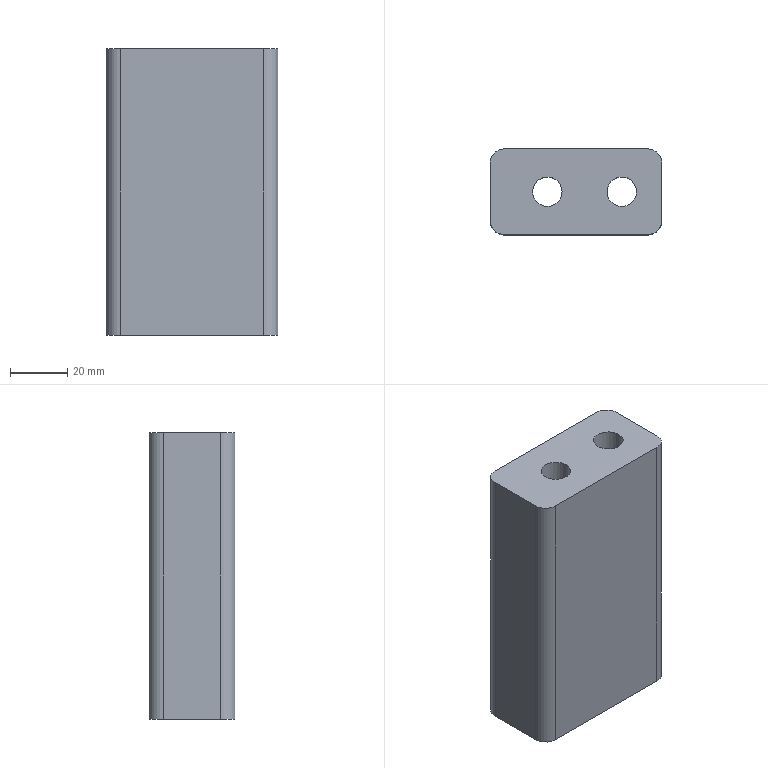Part | NX | features 8 2 | 1 solid | 16 faces | box 60 x 30 x 100 mm | volume 137229 mm3 | plane 8 | cylinder 8 | commonest cylinder face diameters 10 x4 10.3 x2 18 x2
STEP:
#1=CARTESIAN_POINT('',(3731.649,-412.84,91.));
#2=VERTEX_POINT('',#1);
#3=CARTESIAN_POINT('',(3726.499,-412.84,91.));
#4=DIRECTION('',(0.,0.,-1.));
#5=DIRECTION('',(1.,0.,0.));
#6=AXIS2_PLACEMENT_3D('',#3,#4,#5);
#7=CIRCLE('',#6,5.15);
#8=EDGE_CURVE('',#2,#2,#7,.T.);
#9=ORIENTED_EDGE('',*,*,#8,.T.);
#10=EDGE_LOOP('',(#9));
#11=FACE_BOUND('',#10,.T.);
#12=CARTESIAN_POINT('',(3711.499,-397.84,91.));
#13=VERTEX_POINT('',#12);
#14=CARTESIAN_POINT('',(3761.499,-397.84,91.));
#15=VERTEX_POINT('',#14);
#16=CARTESIAN_POINT('',(3721.499,-397.84,91.));
#17=DIRECTION('',(1.,0.,0.));
#18=VECTOR('',#17,1000.);
#19=LINE('',#16,#18);
#20=EDGE_CURVE('',#13,#15,#19,.T.);
#21=ORIENTED_EDGE('',*,*,#20,.F.);
#22=CARTESIAN_POINT('',(3706.499,-402.84,91.));
#23=VERTEX_POINT('',#22);
#24=CARTESIAN_POINT('',(3711.499,-402.84,91.));
#25=DIRECTION('',(0.,0.,1.));
#26=DIRECTION('',(1.,0.,0.));
#27=AXIS2_PLACEMENT_3D('',#24,#25,#26);
#28=CIRCLE('',#27,5.);
#29=EDGE_CURVE('',#13,#23,#28,.T.);
#30=ORIENTED_EDGE('',*,*,#29,.T.);
#31=CARTESIAN_POINT('',(3706.499,-422.84,91.));
#32=VERTEX_POINT('',#31);
#33=CARTESIAN_POINT('',(3706.499,-412.84,91.));
#34=DIRECTION('',(0.,1.,0.));
#35=VECTOR('',#34,1000.);
#36=LINE('',#33,#35);
#37=EDGE_CURVE('',#32,#23,#36,.T.);
#38=ORIENTED_EDGE('',*,*,#37,.F.);
#39=CARTESIAN_POINT('',(3711.499,-427.84,91.));
#40=VERTEX_POINT('',#39);
#41=CARTESIAN_POINT('',(3711.499,-422.84,91.));
#42=DIRECTION('',(0.,0.,1.));
#43=DIRECTION('',(1.,0.,0.));
#44=AXIS2_PLACEMENT_3D('',#41,#42,#43);
#45=CIRCLE('',#44,5.);
#46=EDGE_CURVE('',#32,#40,#45,.T.);
#47=ORIENTED_EDGE('',*,*,#46,.T.);
#48=CARTESIAN_POINT('',(3761.499,-427.84,91.));
#49=VERTEX_POINT('',#48);
#50=CARTESIAN_POINT('',(3721.499,-427.84,91.));
#51=DIRECTION('',(-1.,0.,0.));
#52=VECTOR('',#51,1000.);
#53=LINE('',#50,#52);
#54=EDGE_CURVE('',#49,#40,#53,.T.);
#55=ORIENTED_EDGE('',*,*,#54,.F.);
#56=CARTESIAN_POINT('',(3766.499,-422.84,91.));
#57=VERTEX_POINT('',#56);
#58=CARTESIAN_POINT('',(3761.499,-422.84,91.));
#59=DIRECTION('',(0.,0.,1.));
#60=DIRECTION('',(1.,0.,0.));
#61=AXIS2_PLACEMENT_3D('',#58,#59,#60);
#62=CIRCLE('',#61,5.);
#63=EDGE_CURVE('',#49,#57,#62,.T.);
#64=ORIENTED_EDGE('',*,*,#63,.T.);
#65=CARTESIAN_POINT('',(3766.499,-402.84,91.));
#66=VERTEX_POINT('',#65);
#67=CARTESIAN_POINT('',(3766.499,-412.84,91.));
#68=DIRECTION('',(0.,-1.,0.));
#69=VECTOR('',#68,1000.);
#70=LINE('',#67,#69);
#71=EDGE_CURVE('',#66,#57,#70,.T.);
#72=ORIENTED_EDGE('',*,*,#71,.F.);
#73=CARTESIAN_POINT('',(3761.499,-402.84,91.));
#74=DIRECTION('',(0.,0.,1.));
#75=DIRECTION('',(1.,0.,0.));
#76=AXIS2_PLACEMENT_3D('',#73,#74,#75);
#77=CIRCLE('',#76,5.);
#78=EDGE_CURVE('',#66,#15,#77,.T.);
#79=ORIENTED_EDGE('',*,*,#78,.T.);
#80=EDGE_LOOP('',(#21,#30,#38,#47,#55,#64,#72,#79));
#81=FACE_BOUND('',#80,.T.);
#82=CARTESIAN_POINT('',(3757.649,-412.84,91.));
#83=VERTEX_POINT('',#82);
#84=CARTESIAN_POINT('',(3752.499,-412.84,91.));
#85=DIRECTION('',(0.,0.,-1.));
#86=DIRECTION('',(1.,0.,0.));
#87=AXIS2_PLACEMENT_3D('',#84,#85,#86);
#88=CIRCLE('',#87,5.15);
#89=EDGE_CURVE('',#83,#83,#88,.T.);
#90=ORIENTED_EDGE('',*,*,#89,.T.);
#91=EDGE_LOOP('',(#90));
#92=FACE_BOUND('',#91,.T.);
#93=CARTESIAN_POINT('',(3721.499,-412.84,91.));
#94=DIRECTION('',(0.,0.,1.));
#95=DIRECTION('',(-1.,0.,0.));
#96=AXIS2_PLACEMENT_3D('',#93,#94,#95);
#97=PLANE('',#96);
#98=ADVANCED_FACE('',(#11,#81,#92),#97,.T.);
#99=CARTESIAN_POINT('',(3735.499,-412.84,-9.));
#100=VERTEX_POINT('',#99);
#101=CARTESIAN_POINT('',(3726.499,-412.84,-9.));
#102=DIRECTION('',(0.,0.,1.));
#103=DIRECTION('',(1.,0.,0.));
#104=AXIS2_PLACEMENT_3D('',#101,#102,#103);
#105=CIRCLE('',#104,9.);
#106=EDGE_CURVE('',#100,#100,#105,.T.);
#107=ORIENTED_EDGE('',*,*,#106,.T.);
#108=EDGE_LOOP('',(#107));
#109=FACE_BOUND('',#108,.T.);
#110=CARTESIAN_POINT('',(3706.499,-402.84,-9.));
#111=VERTEX_POINT('',#110);
#112=CARTESIAN_POINT('',(3706.499,-422.84,-9.));
#113=VERTEX_POINT('',#112);
#114=CARTESIAN_POINT('',(3706.499,-412.84,-9.));
#115=DIRECTION('',(0.,-1.,0.));
#116=VECTOR('',#115,1000.);
#117=LINE('',#114,#116);
#118=EDGE_CURVE('',#111,#113,#117,.T.);
#119=ORIENTED_EDGE('',*,*,#118,.F.);
#120=CARTESIAN_POINT('',(3711.499,-397.84,-9.));
#121=VERTEX_POINT('',#120);
#122=CARTESIAN_POINT('',(3711.499,-402.84,-9.));
#123=DIRECTION('',(0.,0.,-1.));
#124=DIRECTION('',(-1.,0.,0.));
#125=AXIS2_PLACEMENT_3D('',#122,#123,#124);
#126=CIRCLE('',#125,5.);
#127=EDGE_CURVE('',#111,#121,#126,.T.);
#128=ORIENTED_EDGE('',*,*,#127,.T.);
#129=CARTESIAN_POINT('',(3761.499,-397.84,-9.));
#130=VERTEX_POINT('',#129);
#131=CARTESIAN_POINT('',(3721.499,-397.84,-9.));
#132=DIRECTION('',(-1.,0.,0.));
#133=VECTOR('',#132,1000.);
#134=LINE('',#131,#133);
#135=EDGE_CURVE('',#130,#121,#134,.T.);
#136=ORIENTED_EDGE('',*,*,#135,.F.);
#137=CARTESIAN_POINT('',(3766.499,-402.84,-9.));
#138=VERTEX_POINT('',#137);
#139=CARTESIAN_POINT('',(3761.499,-402.84,-9.));
#140=DIRECTION('',(0.,0.,-1.));
#141=DIRECTION('',(-1.,0.,0.));
#142=AXIS2_PLACEMENT_3D('',#139,#140,#141);
#143=CIRCLE('',#142,5.);
#144=EDGE_CURVE('',#130,#138,#143,.T.);
#145=ORIENTED_EDGE('',*,*,#144,.T.);
#146=CARTESIAN_POINT('',(3766.499,-422.84,-9.));
#147=VERTEX_POINT('',#146);
#148=CARTESIAN_POINT('',(3766.499,-412.84,-9.));
#149=DIRECTION('',(0.,1.,0.));
#150=VECTOR('',#149,1000.);
#151=LINE('',#148,#150);
#152=EDGE_CURVE('',#147,#138,#151,.T.);
#153=ORIENTED_EDGE('',*,*,#152,.F.);
#154=CARTESIAN_POINT('',(3761.499,-427.84,-9.));
#155=VERTEX_POINT('',#154);
#156=CARTESIAN_POINT('',(3761.499,-422.84,-9.));
#157=DIRECTION('',(0.,0.,-1.));
#158=DIRECTION('',(-1.,0.,0.));
#159=AXIS2_PLACEMENT_3D('',#156,#157,#158);
#160=CIRCLE('',#159,5.);
#161=EDGE_CURVE('',#147,#155,#160,.T.);
#162=ORIENTED_EDGE('',*,*,#161,.T.);
#163=CARTESIAN_POINT('',(3711.499,-427.84,-9.));
#164=VERTEX_POINT('',#163);
#165=CARTESIAN_POINT('',(3721.499,-427.84,-9.));
#166=DIRECTION('',(1.,0.,0.));
#167=VECTOR('',#166,1000.);
#168=LINE('',#165,#167);
#169=EDGE_CURVE('',#164,#155,#168,.T.);
#170=ORIENTED_EDGE('',*,*,#169,.F.);
#171=CARTESIAN_POINT('',(3711.499,-422.84,-9.));
#172=DIRECTION('',(0.,0.,-1.));
#173=DIRECTION('',(-1.,0.,0.));
#174=AXIS2_PLACEMENT_3D('',#171,#172,#173);
#175=CIRCLE('',#174,5.);
#176=EDGE_CURVE('',#164,#113,#175,.T.);
#177=ORIENTED_EDGE('',*,*,#176,.T.);
#178=EDGE_LOOP('',(#119,#128,#136,#145,#153,#162,#170,#177));
#179=FACE_BOUND('',#178,.T.);
#180=CARTESIAN_POINT('',(3761.499,-412.84,-9.));
#181=VERTEX_POINT('',#180);
#182=CARTESIAN_POINT('',(3752.499,-412.84,-9.));
#183=DIRECTION('',(0.,0.,1.));
#184=DIRECTION('',(1.,0.,0.));
#185=AXIS2_PLACEMENT_3D('',#182,#183,#184);
#186=CIRCLE('',#185,9.);
#187=EDGE_CURVE('',#181,#181,#186,.T.);
#188=ORIENTED_EDGE('',*,*,#187,.T.);
#189=EDGE_LOOP('',(#188));
#190=FACE_BOUND('',#189,.T.);
#191=CARTESIAN_POINT('',(3721.499,-412.84,-9.));
#192=DIRECTION('',(0.,0.,-1.));
#193=DIRECTION('',(1.,0.,0.));
#194=AXIS2_PLACEMENT_3D('',#191,#192,#193);
#195=PLANE('',#194);
#196=ADVANCED_FACE('',(#109,#179,#190),#195,.T.);
#197=ORIENTED_EDGE('',*,*,#169,.T.);
#198=CARTESIAN_POINT('',(3761.499,-427.84,-9.));
#199=DIRECTION('',(0.,0.,1.));
#200=VECTOR('',#199,1000.);
#201=LINE('',#198,#200);
#202=EDGE_CURVE('',#155,#49,#201,.T.);
#203=ORIENTED_EDGE('',*,*,#202,.T.);
#204=ORIENTED_EDGE('',*,*,#54,.T.);
#205=CARTESIAN_POINT('',(3711.499,-427.84,-9.));
#206=DIRECTION('',(0.,0.,-1.));
#207=VECTOR('',#206,1000.);
#208=LINE('',#205,#207);
#209=EDGE_CURVE('',#40,#164,#208,.T.);
#210=ORIENTED_EDGE('',*,*,#209,.T.);
#211=EDGE_LOOP('',(#197,#203,#204,#210));
#212=FACE_BOUND('',#211,.T.);
#213=CARTESIAN_POINT('',(3721.499,-427.84,-9.));
#214=DIRECTION('',(0.,-1.,0.));
#215=DIRECTION('',(0.,0.,1.));
#216=AXIS2_PLACEMENT_3D('',#213,#214,#215);
#217=PLANE('',#216);
#218=ADVANCED_FACE('',(#212),#217,.T.);
#219=ORIENTED_EDGE('',*,*,#37,.T.);
#220=CARTESIAN_POINT('',(3706.499,-402.84,-9.));
#221=DIRECTION('',(0.,0.,-1.));
#222=VECTOR('',#221,1000.);
#223=LINE('',#220,#222);
#224=EDGE_CURVE('',#23,#111,#223,.T.);
#225=ORIENTED_EDGE('',*,*,#224,.T.);
#226=ORIENTED_EDGE('',*,*,#118,.T.);
#227=CARTESIAN_POINT('',(3706.499,-422.84,-9.));
#228=DIRECTION('',(0.,0.,1.));
#229=VECTOR('',#228,1000.);
#230=LINE('',#227,#229);
#231=EDGE_CURVE('',#113,#32,#230,.T.);
#232=ORIENTED_EDGE('',*,*,#231,.T.);
#233=EDGE_LOOP('',(#219,#225,#226,#232));
#234=FACE_BOUND('',#233,.T.);
#235=CARTESIAN_POINT('',(3706.499,-412.84,-9.));
#236=DIRECTION('',(-1.,0.,0.));
#237=DIRECTION('',(0.,0.,-1.));
#238=AXIS2_PLACEMENT_3D('',#235,#236,#237);
#239=PLANE('',#238);
#240=ADVANCED_FACE('',(#234),#239,.T.);
#241=ORIENTED_EDGE('',*,*,#135,.T.);
#242=CARTESIAN_POINT('',(3711.499,-397.84,-9.));
#243=DIRECTION('',(0.,0.,1.));
#244=VECTOR('',#243,1000.);
#245=LINE('',#242,#244);
#246=EDGE_CURVE('',#121,#13,#245,.T.);
#247=ORIENTED_EDGE('',*,*,#246,.T.);
#248=ORIENTED_EDGE('',*,*,#20,.T.);
#249=CARTESIAN_POINT('',(3761.499,-397.84,-9.));
#250=DIRECTION('',(0.,0.,-1.));
#251=VECTOR('',#250,1000.);
#252=LINE('',#249,#251);
#253=EDGE_CURVE('',#15,#130,#252,.T.);
#254=ORIENTED_EDGE('',*,*,#253,.T.);
#255=EDGE_LOOP('',(#241,#247,#248,#254));
#256=FACE_BOUND('',#255,.T.);
#257=CARTESIAN_POINT('',(3721.499,-397.84,-9.));
#258=DIRECTION('',(0.,1.,0.));
#259=DIRECTION('',(0.,0.,-1.));
#260=AXIS2_PLACEMENT_3D('',#257,#258,#259);
#261=PLANE('',#260);
#262=ADVANCED_FACE('',(#256),#261,.T.);
#263=ORIENTED_EDGE('',*,*,#152,.T.);
#264=CARTESIAN_POINT('',(3766.499,-402.84,-9.));
#265=DIRECTION('',(0.,0.,1.));
#266=VECTOR('',#265,1000.);
#267=LINE('',#264,#266);
#268=EDGE_CURVE('',#138,#66,#267,.T.);
#269=ORIENTED_EDGE('',*,*,#268,.T.);
#270=ORIENTED_EDGE('',*,*,#71,.T.);
#271=CARTESIAN_POINT('',(3766.499,-422.84,-9.));
#272=DIRECTION('',(0.,0.,-1.));
#273=VECTOR('',#272,1000.);
#274=LINE('',#271,#273);
#275=EDGE_CURVE('',#57,#147,#274,.T.);
#276=ORIENTED_EDGE('',*,*,#275,.T.);
#277=EDGE_LOOP('',(#263,#269,#270,#276));
#278=FACE_BOUND('',#277,.T.);
#279=CARTESIAN_POINT('',(3766.499,-412.84,-9.));
#280=DIRECTION('',(1.,0.,0.));
#281=DIRECTION('',(0.,0.,1.));
#282=AXIS2_PLACEMENT_3D('',#279,#280,#281);
#283=PLANE('',#282);
#284=ADVANCED_FACE('',(#278),#283,.T.);
#285=ORIENTED_EDGE('',*,*,#127,.F.);
#286=ORIENTED_EDGE('',*,*,#224,.F.);
#287=ORIENTED_EDGE('',*,*,#29,.F.);
#288=ORIENTED_EDGE('',*,*,#246,.F.);
#289=EDGE_LOOP('',(#285,#286,#287,#288));
#290=FACE_BOUND('',#289,.T.);
#291=CARTESIAN_POINT('',(3711.499,-402.84,-9.));
#292=DIRECTION('',(0.,0.,1.));
#293=DIRECTION('',(-1.,0.,0.));
#294=AXIS2_PLACEMENT_3D('',#291,#292,#293);
#295=CYLINDRICAL_SURFACE('',#294,5.);
#296=ADVANCED_FACE('',(#290),#295,.T.);
#297=ORIENTED_EDGE('',*,*,#144,.F.);
#298=ORIENTED_EDGE('',*,*,#253,.F.);
#299=ORIENTED_EDGE('',*,*,#78,.F.);
#300=ORIENTED_EDGE('',*,*,#268,.F.);
#301=EDGE_LOOP('',(#297,#298,#299,#300));
#302=FACE_BOUND('',#301,.T.);
#303=CARTESIAN_POINT('',(3761.499,-402.84,-9.));
#304=DIRECTION('',(0.,0.,1.));
#305=DIRECTION('',(-1.,0.,0.));
#306=AXIS2_PLACEMENT_3D('',#303,#304,#305);
#307=CYLINDRICAL_SURFACE('',#306,5.);
#308=ADVANCED_FACE('',(#302),#307,.T.);
#309=ORIENTED_EDGE('',*,*,#161,.F.);
#310=ORIENTED_EDGE('',*,*,#275,.F.);
#311=ORIENTED_EDGE('',*,*,#63,.F.);
#312=ORIENTED_EDGE('',*,*,#202,.F.);
#313=EDGE_LOOP('',(#309,#310,#311,#312));
#314=FACE_BOUND('',#313,.T.);
#315=CARTESIAN_POINT('',(3761.499,-422.84,-9.));
#316=DIRECTION('',(0.,0.,1.));
#317=DIRECTION('',(-1.,0.,0.));
#318=AXIS2_PLACEMENT_3D('',#315,#316,#317);
#319=CYLINDRICAL_SURFACE('',#318,5.);
#320=ADVANCED_FACE('',(#314),#319,.T.);
#321=ORIENTED_EDGE('',*,*,#176,.F.);
#322=ORIENTED_EDGE('',*,*,#209,.F.);
#323=ORIENTED_EDGE('',*,*,#46,.F.);
#324=ORIENTED_EDGE('',*,*,#231,.F.);
#325=EDGE_LOOP('',(#321,#322,#323,#324));
#326=FACE_BOUND('',#325,.T.);
#327=CARTESIAN_POINT('',(3711.499,-422.84,-9.));
#328=DIRECTION('',(0.,0.,1.));
#329=DIRECTION('',(-1.,0.,0.));
#330=AXIS2_PLACEMENT_3D('',#327,#328,#329);
#331=CYLINDRICAL_SURFACE('',#330,5.);
#332=ADVANCED_FACE('',(#326),#331,.T.);
#333=CARTESIAN_POINT('',(3731.649,-412.84,61.));
#334=VERTEX_POINT('',#333);
#335=CARTESIAN_POINT('',(3726.499,-412.84,61.));
#336=DIRECTION('',(0.,0.,1.));
#337=DIRECTION('',(1.,0.,0.));
#338=AXIS2_PLACEMENT_3D('',#335,#336,#337);
#339=CIRCLE('',#338,5.15);
#340=EDGE_CURVE('',#334,#334,#339,.T.);
#341=ORIENTED_EDGE('',*,*,#340,.F.);
#342=EDGE_LOOP('',(#341));
#343=FACE_BOUND('',#342,.T.);
#344=ORIENTED_EDGE('',*,*,#8,.F.);
#345=EDGE_LOOP('',(#344));
#346=FACE_BOUND('',#345,.T.);
#347=CARTESIAN_POINT('',(3726.499,-412.84,-9.));
#348=DIRECTION('',(0.,0.,1.));
#349=DIRECTION('',(-1.,0.,0.));
#350=AXIS2_PLACEMENT_3D('',#347,#348,#349);
#351=CYLINDRICAL_SURFACE('',#350,5.15);
#352=ADVANCED_FACE('',(#343,#346),#351,.F.);
#353=ORIENTED_EDGE('',*,*,#340,.T.);
#354=EDGE_LOOP('',(#353));
#355=FACE_BOUND('',#354,.T.);
#356=CARTESIAN_POINT('',(3735.499,-412.84,61.));
#357=VERTEX_POINT('',#356);
#358=CARTESIAN_POINT('',(3726.499,-412.84,61.));
#359=DIRECTION('',(0.,0.,1.));
#360=DIRECTION('',(1.,0.,0.));
#361=AXIS2_PLACEMENT_3D('',#358,#359,#360);
#362=CIRCLE('',#361,9.);
#363=EDGE_CURVE('',#357,#357,#362,.T.);
#364=ORIENTED_EDGE('',*,*,#363,.F.);
#365=EDGE_LOOP('',(#364));
#366=FACE_BOUND('',#365,.T.);
#367=CARTESIAN_POINT('',(3752.499,-412.84,61.));
#368=DIRECTION('',(0.,0.,1.));
#369=DIRECTION('',(-1.,0.,0.));
#370=AXIS2_PLACEMENT_3D('',#367,#368,#369);
#371=PLANE('',#370);
#372=ADVANCED_FACE('',(#355,#366),#371,.F.);
#373=ORIENTED_EDGE('',*,*,#363,.T.);
#374=EDGE_LOOP('',(#373));
#375=FACE_BOUND('',#374,.T.);
#376=ORIENTED_EDGE('',*,*,#106,.F.);
#377=EDGE_LOOP('',(#376));
#378=FACE_BOUND('',#377,.T.);
#379=CARTESIAN_POINT('',(3726.499,-412.84,-9.));
#380=DIRECTION('',(0.,0.,1.));
#381=DIRECTION('',(-1.,0.,0.));
#382=AXIS2_PLACEMENT_3D('',#379,#380,#381);
#383=CYLINDRICAL_SURFACE('',#382,9.);
#384=ADVANCED_FACE('',(#375,#378),#383,.F.);
#385=CARTESIAN_POINT('',(3757.649,-412.84,61.));
#386=VERTEX_POINT('',#385);
#387=CARTESIAN_POINT('',(3752.499,-412.84,61.));
#388=DIRECTION('',(0.,0.,1.));
#389=DIRECTION('',(1.,0.,0.));
#390=AXIS2_PLACEMENT_3D('',#387,#388,#389);
#391=CIRCLE('',#390,5.15);
#392=EDGE_CURVE('',#386,#386,#391,.T.);
#393=ORIENTED_EDGE('',*,*,#392,.F.);
#394=EDGE_LOOP('',(#393));
#395=FACE_BOUND('',#394,.T.);
#396=ORIENTED_EDGE('',*,*,#89,.F.);
#397=EDGE_LOOP('',(#396));
#398=FACE_BOUND('',#397,.T.);
#399=CARTESIAN_POINT('',(3752.499,-412.84,-9.));
#400=DIRECTION('',(0.,0.,1.));
#401=DIRECTION('',(-1.,0.,0.));
#402=AXIS2_PLACEMENT_3D('',#399,#400,#401);
#403=CYLINDRICAL_SURFACE('',#402,5.15);
#404=ADVANCED_FACE('',(#395,#398),#403,.F.);
#405=ORIENTED_EDGE('',*,*,#392,.T.);
#406=EDGE_LOOP('',(#405));
#407=FACE_BOUND('',#406,.T.);
#408=CARTESIAN_POINT('',(3761.499,-412.84,61.));
#409=VERTEX_POINT('',#408);
#410=CARTESIAN_POINT('',(3752.499,-412.84,61.));
#411=DIRECTION('',(0.,0.,1.));
#412=DIRECTION('',(1.,0.,0.));
#413=AXIS2_PLACEMENT_3D('',#410,#411,#412);
#414=CIRCLE('',#413,9.);
#415=EDGE_CURVE('',#409,#409,#414,.T.);
#416=ORIENTED_EDGE('',*,*,#415,.F.);
#417=EDGE_LOOP('',(#416));
#418=FACE_BOUND('',#417,.T.);
#419=CARTESIAN_POINT('',(3752.499,-412.84,61.));
#420=DIRECTION('',(0.,0.,1.));
#421=DIRECTION('',(-1.,0.,0.));
#422=AXIS2_PLACEMENT_3D('',#419,#420,#421);
#423=PLANE('',#422);
#424=ADVANCED_FACE('',(#407,#418),#423,.F.);
#425=ORIENTED_EDGE('',*,*,#415,.T.);
#426=EDGE_LOOP('',(#425));
#427=FACE_BOUND('',#426,.T.);
#428=ORIENTED_EDGE('',*,*,#187,.F.);
#429=EDGE_LOOP('',(#428));
#430=FACE_BOUND('',#429,.T.);
#431=CARTESIAN_POINT('',(3752.499,-412.84,-9.));
#432=DIRECTION('',(0.,0.,1.));
#433=DIRECTION('',(-1.,0.,0.));
#434=AXIS2_PLACEMENT_3D('',#431,#432,#433);
#435=CYLINDRICAL_SURFACE('',#434,9.);
#436=ADVANCED_FACE('',(#427,#430),#435,.F.);
#437=CLOSED_SHELL('',(#98,#196,#218,#240,#262,#284,#296,#308,#320,#332,#352,#372,#384,#404,#424,#436));
#438=MANIFOLD_SOLID_BREP('',#437);
#439=(LENGTH_UNIT()NAMED_UNIT(*)SI_UNIT(.MILLI.,.METRE.));
#440=UNCERTAINTY_MEASURE_WITH_UNIT(LENGTH_MEASURE(0.00001),#439,'','');
#441=(NAMED_UNIT(*)PLANE_ANGLE_UNIT()SI_UNIT($,.RADIAN.));
#442=(NAMED_UNIT(*)SI_UNIT($,.STERADIAN.)SOLID_ANGLE_UNIT());
#443=(GEOMETRIC_REPRESENTATION_CONTEXT(3)GLOBAL_UNCERTAINTY_ASSIGNED_CONTEXT((#440))GLOBAL_UNIT_ASSIGNED_CONTEXT((#439,#441,#442))REPRESENTATION_CONTEXT('',''));
#444=ADVANCED_BREP_SHAPE_REPRESENTATION('',(#438),#443);